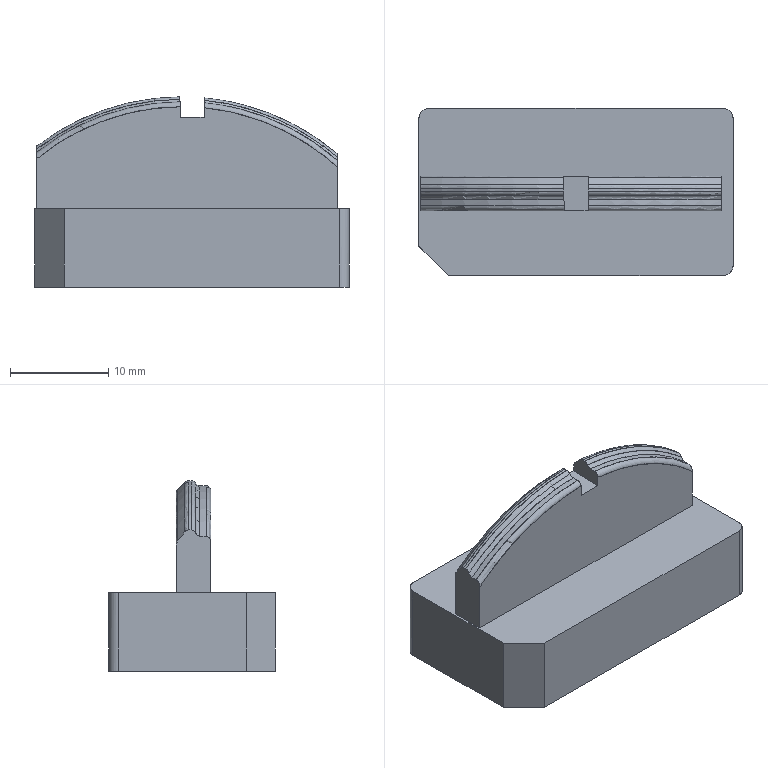CAM job | PowerMill | 3-axis milling, other | part box 32 x 17 x 19.383 mm
Tools:
number,name,type,diameter,tip_radius,length,cutting_length,overhang,flutes,holder,toolpaths_using
1,D10C,end_mill,10.0,0.0,60.0,,30.0,1,D42L35,1
2,D4C,end_mill,4.0,0.0,30.0,,15.0,1,D42L35,1
1,D10C_1_1_1,end_mill,10.0,0.0,60.0,,19.84,1,D42L35,3
2,D4C_1_1,end_mill,4.0,0.0,30.0,,11.56,1,D42L35,1
28,D2C_1_1,end_mill,2.0,0.0,3.0,,2.36,1,D42L35,1
3,D10_1_1_1,end_mill,10.0,0.0,60.0,,19.56,1,D42L35,3
22,R1.5_1_1,ball_nosed,3.0,1.5,30.0,,9.0,1,D42L35,1
6,R0.5_1_1,ball_nosed,1.0,0.5,3.0,,7.08,1,D42L35,1
12,D2_1_1,end_mill,2.0,0.0,3.0,,2.48,1,D42L35,1
13,Text_D4_1_1,taper_spherical,4.0,0.3,60.0,,11.64,1,D42L35,1
Operations:
program,toolpath,strategy,tool,tool_number,tool_diameter,tip_radius,flutes,spindle_rpm,feed_cut,surface_speed_m_min_computed,feed_per_tooth_computed,tolerance,thickness,stepover,stepdown,cut_length,cut_time_min,total_time_min,workplane
19-B01-19-F,精公开粗01-扫面平行-D10C,raster_area_clear,D10C_1_1_1,1,10.0,0.0,1.0,8000.0,10000.0,251.33,1.25,0.03,0.28,6.0,1.0,210.36,0.021,0.0268,
19-B01-19-F,精公开粗01-外形偏置-D10C,offset_area_clear,D10C_1_1_1,1,10.0,0.0,1.0,8000.0,10000.0,251.33,1.25,0.03,0.28,6.0,1.0,7004.066,0.7,0.7731,
19-B01-19-F,精公开粗01-基准台等高-D10C,constantz,D10C_1_1_1,1,10.0,0.0,1.0,8000.0,10000.0,251.33,1.25,0.03,0.07,5.0,0.4,2789.036,0.279,0.2887,
19-B01-19-F,精公再粗02-外形偏置-D4C,offset_area_clear,D4C_1_1,2,4.0,0.0,1.0,18000.0,6000.0,226.19,0.3333,0.03,0.0,2.0,1.0,4223.644,0.704,0.7338,
19-B01-19-F,精公再粗03-外形偏置-D2C,offset_area_clear,D2C_1_1,28,2.0,0.0,1.0,18000.0,4000.0,113.1,0.2222,0.03,0.0,1.1,1.0,202.689,0.051,0.0783,
19-B01-19-F,精公基准台01-基准面偏置-D10,offset_area_clear,D10_1_1_1,3,10.0,0.0,1.0,8500.0,600.0,267.04,0.0706,0.005,0.38,5.0,1.0,111.472,0.186,0.2049,
19-B01-19-F,精公基准台01-外形侧光-D10,profile_area_clear,D10_1_1_1,3,10.0,0.0,1.0,8500.0,600.0,267.04,0.0706,0.005,-0.07,0.08,1.0,198.963,0.332,0.3524,
19-B01-19-F,精公基准台01-基准台侧光-D10,profile_area_clear,D10_1_1_1,3,10.0,0.0,1.0,8500.0,600.0,267.04,0.0706,0.005,0.0,0.08,1.0,253.233,0.422,0.4863,
19-B01-19-F,精公精光01-平行-R1.5,raster,R1.5_1_1,22,3.0,1.5,1.0,22000.0,2000.0,207.35,0.0909,0.005,-0.075,0.04,1.0,6354.397,3.177,3.21,
19-B01-19-F,精公精光02-清角-R0.5,automatic_corner,R0.5_1_1,6,1.0,0.5,1.0,20000.0,1000.0,62.83,0.05,0.005,-0.075,5.0,1.0,1582.392,1.582,1.636,
19-B01-19-F,精公精光03-等高-D2,constantz,D2_1_1,12,2.0,0.0,1.0,18000.0,1500.0,113.1,0.0833,0.005,-0.075,5.0,0.03,533.811,0.356,0.4631,
19-B01-19-F,精公刻字01-刻字-Text_D4,pattern,Text_D4_1_1,13,4.0,0.3,1.0,15000.0,1000.0,188.5,0.0667,0.005,0.0,5.0,1.0,54.35,0.054,0.0747,
,精公开粗01-外形偏置-D10C_Reference,offset_area_clear,D10C,1,10.0,0.0,1.0,8000.0,10000.0,251.33,1.25,0.03,0.28,6.0,1.0,13822.244,1.382,1.523,
,精公再粗02-外形偏置-D4C_Reference,offset_area_clear,D4C,2,4.0,0.0,1.0,18000.0,6000.0,226.19,0.3333,0.03,0.0,2.0,1.0,8271.224,1.379,1.428,